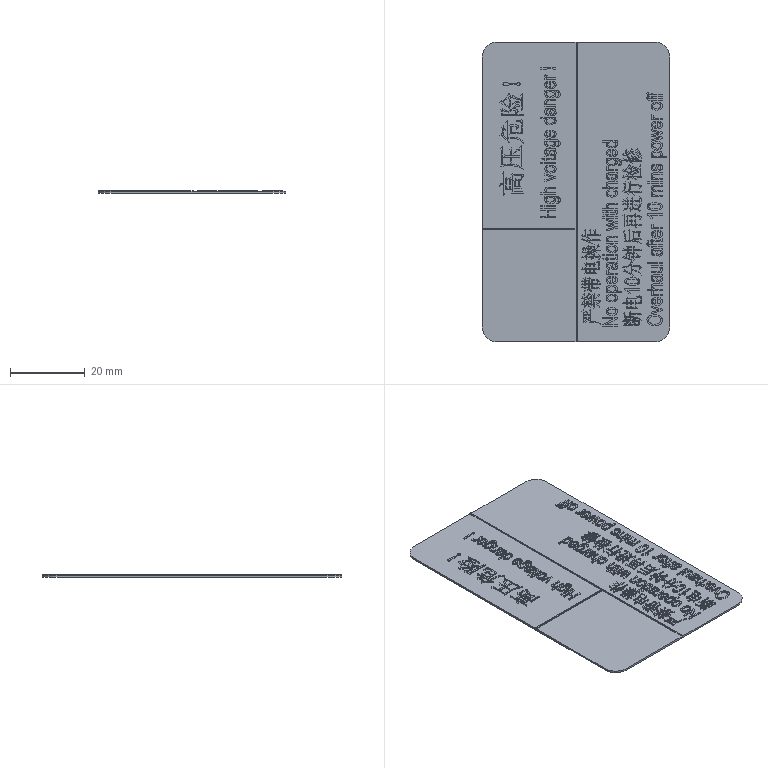Part | SolidWorks | features BaseBody 1 | 1 solid | 1754 faces | box 50 x 80 x 0.7 mm | volume 2057 mm3 | plane 1210 | spline 540 | cylinder 4 | commonest cylinder face diameters 8 x4